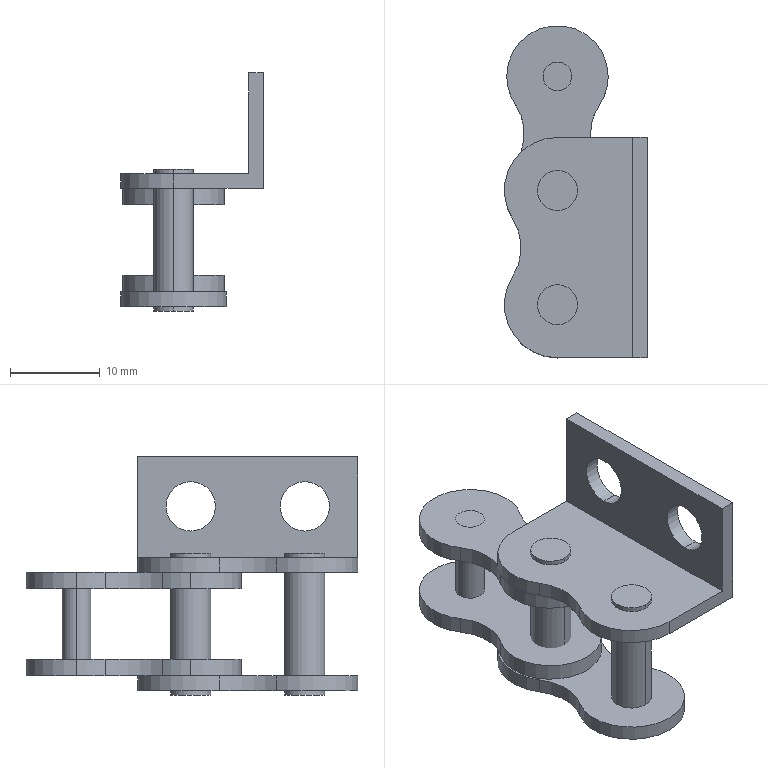Part | STEP file | 08b-1_e-1k2v1V11 | 4 solids | 71 faces | box 15.9 x 36.944 x 26.5 mm | volume 2584 mm3 | cylinder 52 | plane 19 | commonest cylinder face diameters 11.289 x18 4.45 x12 3.191 x10 11.8 x8 5.5 x4